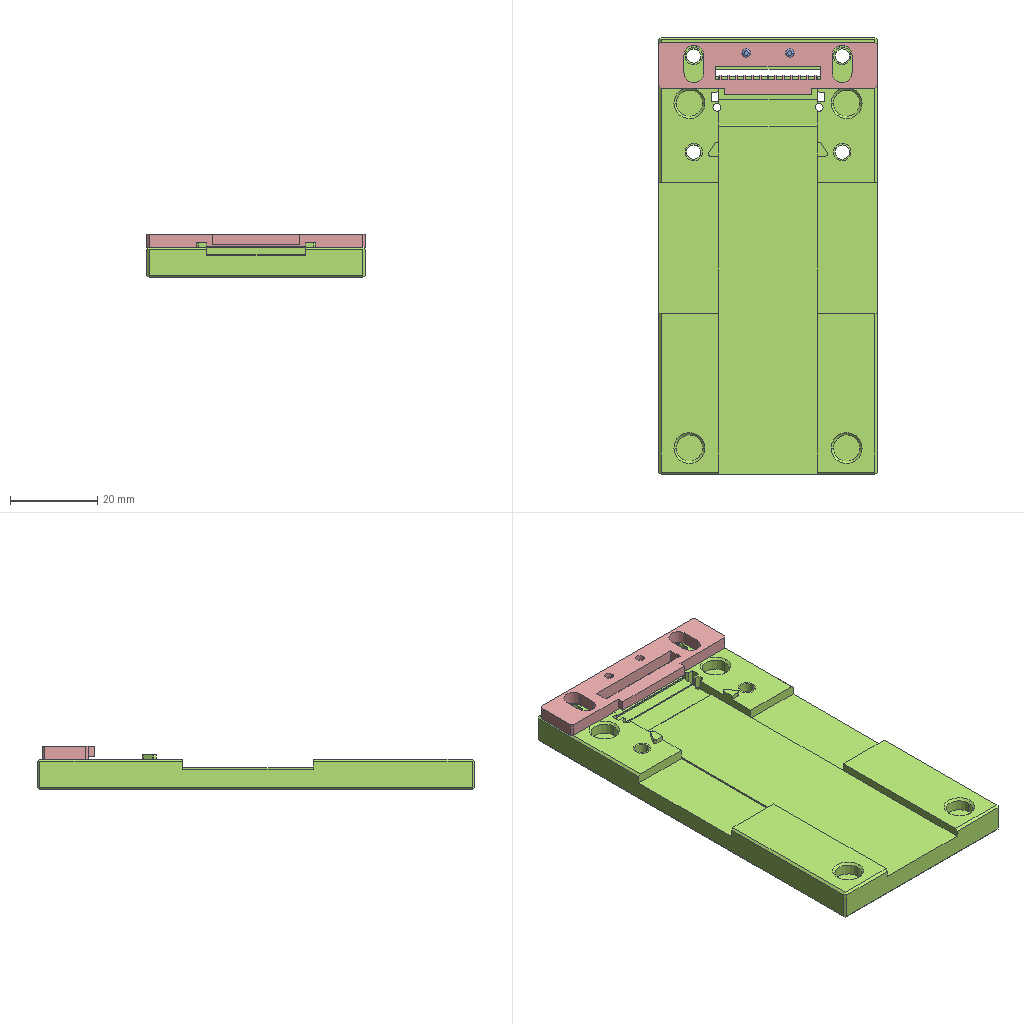Assembly | SolidWorks | 8 different items | 9 placed | box 50 x 100 x 10 mm
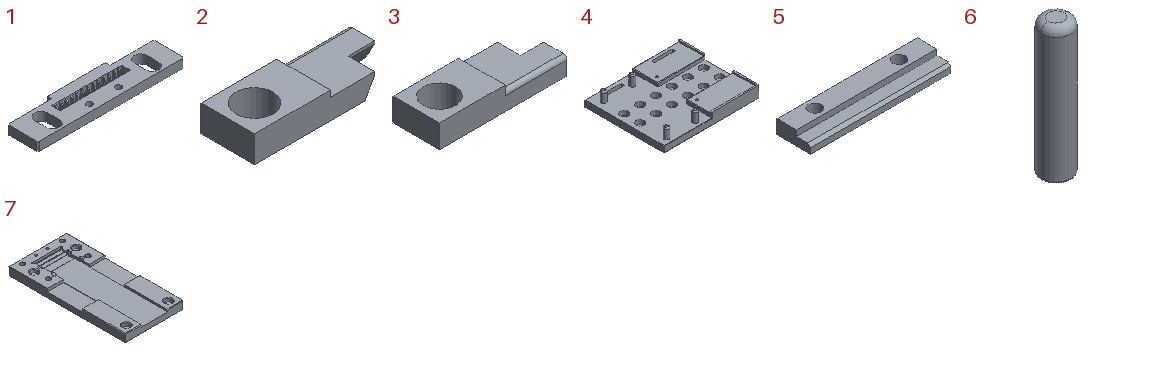Parts list (item | name | quantity | size | volume | features):
1 | - | x1 | 50 x 12 x 3 mm | 1210 mm3 | features BaseBody 1, HoleWzd 1
2 | - | x1 | 16.5 x 6 x 3 mm | 192.89 mm3 | features BaseBody 1
3 | - | x1 | 16.5 x 6 x 3 mm | 192.89 mm3 | features BaseBody 1
4 | - | x1 | 120 x 100 x 21 mm | 106763 mm3 | features BaseBody 1
5 | - | x1 | 50 x 12 x 5 mm | 2316 mm3 | features BaseBody 1
6 | - | x2 | 2 x 2 x 9 mm | 27.962 mm3 | features Fillet 2, Extrusion 1
7 | - | x1 | - | - | features RefSurface 4, BaseBody 1, HoleWzd 1
8 | JXN-PADLESS-ZZ007 | x1 | - | - | -
Mates (type | each side: item.copy, entity, surface, feature):
Coincident | 7.1 face plane Input1 | 1.1 face plane Input1 | 2 times
DistanceDim | 7.1 face plane Input1 | 1.1 face plane Input1
Coincident | 4.1 face plane Input1 | 6.1 face plane Boss-Extrude1
Concentric | 7.1 face cylinder Ø2.0 (2) Diameter Hole1 | 6.1 face cylinder Boss-Extrude1
Coincident | 4.1 face plane Input1 | 6.2 face plane Boss-Extrude1
Concentric | 7.1 face cylinder Ø2.0 (2) Diameter Hole1 | 6.2 face cylinder Boss-Extrude1